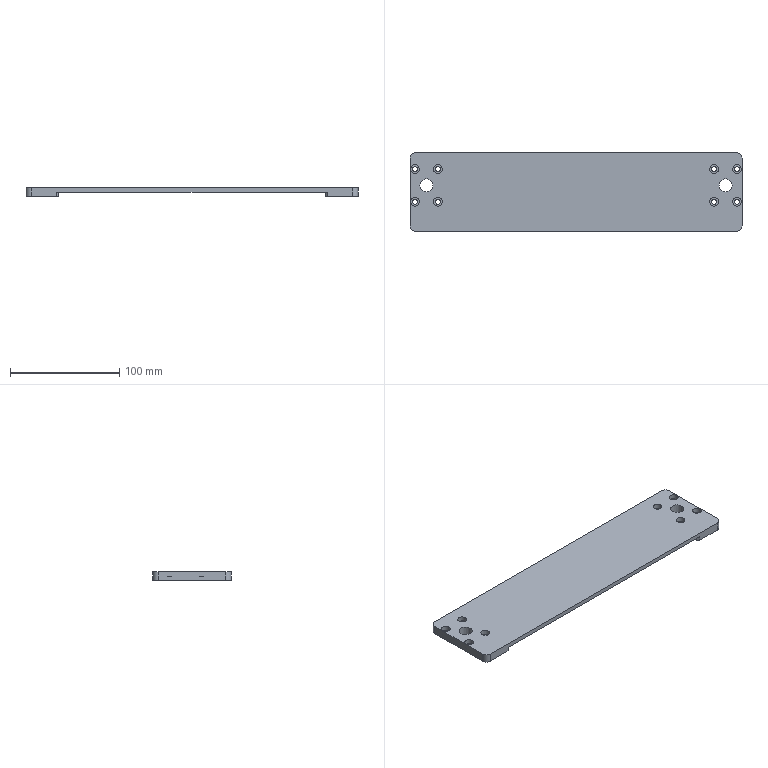Part | NX | 1 solid | 44 faces | box 304 x 72 x 8 mm | volume 100591 mm3 | plane 22 | cylinder 22 | commonest cylinder face diameters 4.5 x8 8 x8 10 x4 12 x2
STEP:
#1=CARTESIAN_POINT('',(151.5,-9.,-0.4));
#2=VERTEX_POINT('',#1);
#3=CARTESIAN_POINT('',(147.5,-9.,-0.4));
#4=DIRECTION('',(0.,0.,1.));
#5=DIRECTION('',(1.,0.,0.));
#6=AXIS2_PLACEMENT_3D('',#3,#4,#5);
#7=CIRCLE('',#6,4.);
#8=EDGE_CURVE('',#2,#2,#7,.T.);
#9=ORIENTED_EDGE('',*,*,#8,.T.);
#10=EDGE_LOOP('',(#9));
#11=FACE_BOUND('',#10,.T.);
#12=CARTESIAN_POINT('',(149.75,-9.,-0.4));
#13=VERTEX_POINT('',#12);
#14=CARTESIAN_POINT('',(147.5,-9.,-0.4));
#15=DIRECTION('',(0.,0.,1.));
#16=DIRECTION('',(1.,0.,0.));
#17=AXIS2_PLACEMENT_3D('',#14,#15,#16);
#18=CIRCLE('',#17,2.25);
#19=EDGE_CURVE('',#13,#13,#18,.T.);
#20=ORIENTED_EDGE('',*,*,#19,.F.);
#21=EDGE_LOOP('',(#20));
#22=FACE_BOUND('',#21,.T.);
#23=CARTESIAN_POINT('',(149.75,-9.,-0.4));
#24=DIRECTION('',(0.,0.,-1.));
#25=DIRECTION('',(-1.,0.,0.));
#26=AXIS2_PLACEMENT_3D('',#23,#24,#25);
#27=PLANE('',#26);
#28=ADVANCED_FACE('',(#11,#22),#27,.F.);
#29=CARTESIAN_POINT('',(143.5,21.,-0.4));
#30=VERTEX_POINT('',#29);
#31=CARTESIAN_POINT('',(147.5,21.,-0.4));
#32=DIRECTION('',(0.,0.,1.));
#33=DIRECTION('',(-1.,0.,0.));
#34=AXIS2_PLACEMENT_3D('',#31,#32,#33);
#35=CIRCLE('',#34,4.);
#36=EDGE_CURVE('',#30,#30,#35,.T.);
#37=ORIENTED_EDGE('',*,*,#36,.T.);
#38=EDGE_LOOP('',(#37));
#39=FACE_BOUND('',#38,.T.);
#40=CARTESIAN_POINT('',(145.25,21.,-0.4));
#41=VERTEX_POINT('',#40);
#42=CARTESIAN_POINT('',(147.5,21.,-0.4));
#43=DIRECTION('',(0.,0.,1.));
#44=DIRECTION('',(-1.,0.,0.));
#45=AXIS2_PLACEMENT_3D('',#42,#43,#44);
#46=CIRCLE('',#45,2.25);
#47=EDGE_CURVE('',#41,#41,#46,.T.);
#48=ORIENTED_EDGE('',*,*,#47,.F.);
#49=EDGE_LOOP('',(#48));
#50=FACE_BOUND('',#49,.T.);
#51=CARTESIAN_POINT('',(149.75,-9.,-0.4));
#52=DIRECTION('',(0.,0.,-1.));
#53=DIRECTION('',(-1.,0.,0.));
#54=AXIS2_PLACEMENT_3D('',#51,#52,#53);
#55=PLANE('',#54);
#56=ADVANCED_FACE('',(#39,#50),#55,.F.);
#57=CARTESIAN_POINT('',(122.5,21.,-0.4));
#58=VERTEX_POINT('',#57);
#59=CARTESIAN_POINT('',(126.5,21.,-0.4));
#60=DIRECTION('',(0.,0.,1.));
#61=DIRECTION('',(-1.,0.,0.));
#62=AXIS2_PLACEMENT_3D('',#59,#60,#61);
#63=CIRCLE('',#62,4.);
#64=EDGE_CURVE('',#58,#58,#63,.T.);
#65=ORIENTED_EDGE('',*,*,#64,.T.);
#66=EDGE_LOOP('',(#65));
#67=FACE_BOUND('',#66,.T.);
#68=CARTESIAN_POINT('',(124.25,21.,-0.4));
#69=VERTEX_POINT('',#68);
#70=CARTESIAN_POINT('',(126.5,21.,-0.4));
#71=DIRECTION('',(0.,0.,1.));
#72=DIRECTION('',(-1.,0.,0.));
#73=AXIS2_PLACEMENT_3D('',#70,#71,#72);
#74=CIRCLE('',#73,2.25);
#75=EDGE_CURVE('',#69,#69,#74,.T.);
#76=ORIENTED_EDGE('',*,*,#75,.F.);
#77=EDGE_LOOP('',(#76));
#78=FACE_BOUND('',#77,.T.);
#79=CARTESIAN_POINT('',(149.75,-9.,-0.4));
#80=DIRECTION('',(0.,0.,-1.));
#81=DIRECTION('',(-1.,0.,0.));
#82=AXIS2_PLACEMENT_3D('',#79,#80,#81);
#83=PLANE('',#82);
#84=ADVANCED_FACE('',(#67,#78),#83,.F.);
#85=CARTESIAN_POINT('',(122.5,-9.,-0.4));
#86=VERTEX_POINT('',#85);
#87=CARTESIAN_POINT('',(126.5,-9.,-0.4));
#88=DIRECTION('',(0.,0.,1.));
#89=DIRECTION('',(-1.,0.,0.));
#90=AXIS2_PLACEMENT_3D('',#87,#88,#89);
#91=CIRCLE('',#90,4.);
#92=EDGE_CURVE('',#86,#86,#91,.T.);
#93=ORIENTED_EDGE('',*,*,#92,.T.);
#94=EDGE_LOOP('',(#93));
#95=FACE_BOUND('',#94,.T.);
#96=CARTESIAN_POINT('',(124.25,-9.,-0.4));
#97=VERTEX_POINT('',#96);
#98=CARTESIAN_POINT('',(126.5,-9.,-0.4));
#99=DIRECTION('',(0.,0.,1.));
#100=DIRECTION('',(-1.,0.,0.));
#101=AXIS2_PLACEMENT_3D('',#98,#99,#100);
#102=CIRCLE('',#101,2.25);
#103=EDGE_CURVE('',#97,#97,#102,.T.);
#104=ORIENTED_EDGE('',*,*,#103,.F.);
#105=EDGE_LOOP('',(#104));
#106=FACE_BOUND('',#105,.T.);
#107=CARTESIAN_POINT('',(149.75,-9.,-0.4));
#108=DIRECTION('',(0.,0.,-1.));
#109=DIRECTION('',(-1.,0.,0.));
#110=AXIS2_PLACEMENT_3D('',#107,#108,#109);
#111=PLANE('',#110);
#112=ADVANCED_FACE('',(#95,#106),#111,.F.);
#113=CARTESIAN_POINT('',(-130.5,-9.,-0.4));
#114=VERTEX_POINT('',#113);
#115=CARTESIAN_POINT('',(-126.5,-9.,-0.4));
#116=DIRECTION('',(0.,0.,1.));
#117=DIRECTION('',(-1.,0.,0.));
#118=AXIS2_PLACEMENT_3D('',#115,#116,#117);
#119=CIRCLE('',#118,4.);
#120=EDGE_CURVE('',#114,#114,#119,.T.);
#121=ORIENTED_EDGE('',*,*,#120,.T.);
#122=EDGE_LOOP('',(#121));
#123=FACE_BOUND('',#122,.T.);
#124=CARTESIAN_POINT('',(-128.75,-9.,-0.4));
#125=VERTEX_POINT('',#124);
#126=CARTESIAN_POINT('',(-126.5,-9.,-0.4));
#127=DIRECTION('',(0.,0.,1.));
#128=DIRECTION('',(-1.,0.,0.));
#129=AXIS2_PLACEMENT_3D('',#126,#127,#128);
#130=CIRCLE('',#129,2.25);
#131=EDGE_CURVE('',#125,#125,#130,.T.);
#132=ORIENTED_EDGE('',*,*,#131,.F.);
#133=EDGE_LOOP('',(#132));
#134=FACE_BOUND('',#133,.T.);
#135=CARTESIAN_POINT('',(149.75,-9.,-0.4));
#136=DIRECTION('',(0.,0.,-1.));
#137=DIRECTION('',(-1.,0.,0.));
#138=AXIS2_PLACEMENT_3D('',#135,#136,#137);
#139=PLANE('',#138);
#140=ADVANCED_FACE('',(#123,#134),#139,.F.);
#141=CARTESIAN_POINT('',(-130.5,21.,-0.4));
#142=VERTEX_POINT('',#141);
#143=CARTESIAN_POINT('',(-126.5,21.,-0.4));
#144=DIRECTION('',(0.,0.,1.));
#145=DIRECTION('',(-1.,0.,0.));
#146=AXIS2_PLACEMENT_3D('',#143,#144,#145);
#147=CIRCLE('',#146,4.);
#148=EDGE_CURVE('',#142,#142,#147,.T.);
#149=ORIENTED_EDGE('',*,*,#148,.T.);
#150=EDGE_LOOP('',(#149));
#151=FACE_BOUND('',#150,.T.);
#152=CARTESIAN_POINT('',(-128.75,21.,-0.4));
#153=VERTEX_POINT('',#152);
#154=CARTESIAN_POINT('',(-126.5,21.,-0.4));
#155=DIRECTION('',(0.,0.,1.));
#156=DIRECTION('',(-1.,0.,0.));
#157=AXIS2_PLACEMENT_3D('',#154,#155,#156);
#158=CIRCLE('',#157,2.25);
#159=EDGE_CURVE('',#153,#153,#158,.T.);
#160=ORIENTED_EDGE('',*,*,#159,.F.);
#161=EDGE_LOOP('',(#160));
#162=FACE_BOUND('',#161,.T.);
#163=CARTESIAN_POINT('',(149.75,-9.,-0.4));
#164=DIRECTION('',(0.,0.,-1.));
#165=DIRECTION('',(-1.,0.,0.));
#166=AXIS2_PLACEMENT_3D('',#163,#164,#165);
#167=PLANE('',#166);
#168=ADVANCED_FACE('',(#151,#162),#167,.F.);
#169=CARTESIAN_POINT('',(-151.5,21.,-0.4));
#170=VERTEX_POINT('',#169);
#171=CARTESIAN_POINT('',(-147.5,21.,-0.4));
#172=DIRECTION('',(0.,0.,1.));
#173=DIRECTION('',(-1.,0.,0.));
#174=AXIS2_PLACEMENT_3D('',#171,#172,#173);
#175=CIRCLE('',#174,4.);
#176=EDGE_CURVE('',#170,#170,#175,.T.);
#177=ORIENTED_EDGE('',*,*,#176,.T.);
#178=EDGE_LOOP('',(#177));
#179=FACE_BOUND('',#178,.T.);
#180=CARTESIAN_POINT('',(-149.75,21.,-0.4));
#181=VERTEX_POINT('',#180);
#182=CARTESIAN_POINT('',(-147.5,21.,-0.4));
#183=DIRECTION('',(0.,0.,1.));
#184=DIRECTION('',(-1.,0.,0.));
#185=AXIS2_PLACEMENT_3D('',#182,#183,#184);
#186=CIRCLE('',#185,2.25);
#187=EDGE_CURVE('',#181,#181,#186,.T.);
#188=ORIENTED_EDGE('',*,*,#187,.F.);
#189=EDGE_LOOP('',(#188));
#190=FACE_BOUND('',#189,.T.);
#191=CARTESIAN_POINT('',(149.75,-9.,-0.4));
#192=DIRECTION('',(0.,0.,-1.));
#193=DIRECTION('',(-1.,0.,0.));
#194=AXIS2_PLACEMENT_3D('',#191,#192,#193);
#195=PLANE('',#194);
#196=ADVANCED_FACE('',(#179,#190),#195,.F.);
#197=CARTESIAN_POINT('',(-151.5,-9.,-0.4));
#198=VERTEX_POINT('',#197);
#199=CARTESIAN_POINT('',(-147.5,-9.,-0.4));
#200=DIRECTION('',(0.,0.,1.));
#201=DIRECTION('',(-1.,0.,0.));
#202=AXIS2_PLACEMENT_3D('',#199,#200,#201);
#203=CIRCLE('',#202,4.);
#204=EDGE_CURVE('',#198,#198,#203,.T.);
#205=ORIENTED_EDGE('',*,*,#204,.T.);
#206=EDGE_LOOP('',(#205));
#207=FACE_BOUND('',#206,.T.);
#208=CARTESIAN_POINT('',(-149.75,-9.,-0.4));
#209=VERTEX_POINT('',#208);
#210=CARTESIAN_POINT('',(-147.5,-9.,-0.4));
#211=DIRECTION('',(0.,0.,1.));
#212=DIRECTION('',(-1.,0.,0.));
#213=AXIS2_PLACEMENT_3D('',#210,#211,#212);
#214=CIRCLE('',#213,2.25);
#215=EDGE_CURVE('',#209,#209,#214,.T.);
#216=ORIENTED_EDGE('',*,*,#215,.F.);
#217=EDGE_LOOP('',(#216));
#218=FACE_BOUND('',#217,.T.);
#219=CARTESIAN_POINT('',(149.75,-9.,-0.4));
#220=DIRECTION('',(0.,0.,-1.));
#221=DIRECTION('',(-1.,0.,0.));
#222=AXIS2_PLACEMENT_3D('',#219,#220,#221);
#223=PLANE('',#222);
#224=ADVANCED_FACE('',(#207,#218),#223,.F.);
#225=CARTESIAN_POINT('',(-124.,-36.,0.));
#226=VERTEX_POINT('',#225);
#227=CARTESIAN_POINT('',(-122.,-34.,0.));
#228=VERTEX_POINT('',#227);
#229=CARTESIAN_POINT('',(-122.,-34.,0.));
#230=DIRECTION('',(0.7071,0.7071,0.));
#231=VECTOR('',#230,1000.);
#232=LINE('',#229,#231);
#233=EDGE_CURVE('',#226,#228,#232,.T.);
#234=ORIENTED_EDGE('',*,*,#233,.F.);
#235=CARTESIAN_POINT('',(-124.,-36.,-4.));
#236=VERTEX_POINT('',#235);
#237=CARTESIAN_POINT('',(-124.,-36.,4.));
#238=DIRECTION('',(0.,0.,1.));
#239=VECTOR('',#238,1000.);
#240=LINE('',#237,#239);
#241=EDGE_CURVE('',#236,#226,#240,.T.);
#242=ORIENTED_EDGE('',*,*,#241,.F.);
#243=CARTESIAN_POINT('',(-122.,-34.,-4.));
#244=VERTEX_POINT('',#243);
#245=CARTESIAN_POINT('',(-122.,-34.,-4.));
#246=DIRECTION('',(-0.7071,-0.7071,0.));
#247=VECTOR('',#246,1000.);
#248=LINE('',#245,#247);
#249=EDGE_CURVE('',#244,#236,#248,.T.);
#250=ORIENTED_EDGE('',*,*,#249,.F.);
#251=CARTESIAN_POINT('',(-122.,-34.,0.));
#252=DIRECTION('',(0.,0.,-1.));
#253=VECTOR('',#252,1000.);
#254=LINE('',#251,#253);
#255=EDGE_CURVE('',#228,#244,#254,.T.);
#256=ORIENTED_EDGE('',*,*,#255,.F.);
#257=EDGE_LOOP('',(#234,#242,#250,#256));
#258=FACE_BOUND('',#257,.T.);
#259=CARTESIAN_POINT('',(-122.,-34.,0.));
#260=DIRECTION('',(-0.7071,0.7071,0.));
#261=DIRECTION('',(0.,0.,-1.));
#262=AXIS2_PLACEMENT_3D('',#259,#260,#261);
#263=PLANE('',#262);
#264=ADVANCED_FACE('',(#258),#263,.F.);
#265=CARTESIAN_POINT('',(-122.,34.,0.));
#266=VERTEX_POINT('',#265);
#267=CARTESIAN_POINT('',(-124.,36.,0.));
#268=VERTEX_POINT('',#267);
#269=CARTESIAN_POINT('',(-124.,36.,0.));
#270=DIRECTION('',(-0.7071,0.7071,0.));
#271=VECTOR('',#270,1000.);
#272=LINE('',#269,#271);
#273=EDGE_CURVE('',#266,#268,#272,.T.);
#274=ORIENTED_EDGE('',*,*,#273,.F.);
#275=CARTESIAN_POINT('',(-122.,34.,-4.));
#276=VERTEX_POINT('',#275);
#277=CARTESIAN_POINT('',(-122.,34.,0.));
#278=DIRECTION('',(0.,0.,1.));
#279=VECTOR('',#278,1000.);
#280=LINE('',#277,#279);
#281=EDGE_CURVE('',#276,#266,#280,.T.);
#282=ORIENTED_EDGE('',*,*,#281,.F.);
#283=CARTESIAN_POINT('',(-124.,36.,-4.));
#284=VERTEX_POINT('',#283);
#285=CARTESIAN_POINT('',(-124.,36.,-4.));
#286=DIRECTION('',(0.7071,-0.7071,0.));
#287=VECTOR('',#286,1000.);
#288=LINE('',#285,#287);
#289=EDGE_CURVE('',#284,#276,#288,.T.);
#290=ORIENTED_EDGE('',*,*,#289,.F.);
#291=CARTESIAN_POINT('',(-124.,36.,4.));
#292=DIRECTION('',(0.,0.,-1.));
#293=VECTOR('',#292,1000.);
#294=LINE('',#291,#293);
#295=EDGE_CURVE('',#268,#284,#294,.T.);
#296=ORIENTED_EDGE('',*,*,#295,.F.);
#297=EDGE_LOOP('',(#274,#282,#290,#296));
#298=FACE_BOUND('',#297,.T.);
#299=CARTESIAN_POINT('',(-124.,36.,4.));
#300=DIRECTION('',(-0.7071,-0.7071,0.));
#301=DIRECTION('',(0.,0.,-1.));
#302=AXIS2_PLACEMENT_3D('',#299,#300,#301);
#303=PLANE('',#302);
#304=ADVANCED_FACE('',(#298),#303,.F.);
#305=CARTESIAN_POINT('',(122.,-34.,0.));
#306=VERTEX_POINT('',#305);
#307=CARTESIAN_POINT('',(124.,-36.,0.));
#308=VERTEX_POINT('',#307);
#309=CARTESIAN_POINT('',(124.,-36.,0.));
#310=DIRECTION('',(0.7071,-0.7071,0.));
#311=VECTOR('',#310,1000.);
#312=LINE('',#309,#311);
#313=EDGE_CURVE('',#306,#308,#312,.T.);
#314=ORIENTED_EDGE('',*,*,#313,.F.);
#315=CARTESIAN_POINT('',(122.,-34.,-4.));
#316=VERTEX_POINT('',#315);
#317=CARTESIAN_POINT('',(122.,-34.,0.));
#318=DIRECTION('',(0.,0.,1.));
#319=VECTOR('',#318,1000.);
#320=LINE('',#317,#319);
#321=EDGE_CURVE('',#316,#306,#320,.T.);
#322=ORIENTED_EDGE('',*,*,#321,.F.);
#323=CARTESIAN_POINT('',(124.,-36.,-4.));
#324=VERTEX_POINT('',#323);
#325=CARTESIAN_POINT('',(124.,-36.,-4.));
#326=DIRECTION('',(-0.7071,0.7071,0.));
#327=VECTOR('',#326,1000.);
#328=LINE('',#325,#327);
#329=EDGE_CURVE('',#324,#316,#328,.T.);
#330=ORIENTED_EDGE('',*,*,#329,.F.);
#331=CARTESIAN_POINT('',(124.,-36.,4.));
#332=DIRECTION('',(0.,0.,-1.));
#333=VECTOR('',#332,1000.);
#334=LINE('',#331,#333);
#335=EDGE_CURVE('',#308,#324,#334,.T.);
#336=ORIENTED_EDGE('',*,*,#335,.F.);
#337=EDGE_LOOP('',(#314,#322,#330,#336));
#338=FACE_BOUND('',#337,.T.);
#339=CARTESIAN_POINT('',(124.,-36.,4.));
#340=DIRECTION('',(0.7071,0.7071,0.));
#341=DIRECTION('',(0.,0.,-1.));
#342=AXIS2_PLACEMENT_3D('',#339,#340,#341);
#343=PLANE('',#342);
#344=ADVANCED_FACE('',(#338),#343,.F.);
#345=CARTESIAN_POINT('',(124.,36.,0.));
#346=VERTEX_POINT('',#345);
#347=CARTESIAN_POINT('',(122.,34.,0.));
#348=VERTEX_POINT('',#347);
#349=CARTESIAN_POINT('',(122.,34.,0.));
#350=DIRECTION('',(-0.7071,-0.7071,0.));
#351=VECTOR('',#350,1000.);
#352=LINE('',#349,#351);
#353=EDGE_CURVE('',#346,#348,#352,.T.);
#354=ORIENTED_EDGE('',*,*,#353,.F.);
#355=CARTESIAN_POINT('',(124.,36.,-4.));
#356=VERTEX_POINT('',#355);
#357=CARTESIAN_POINT('',(124.,36.,4.));
#358=DIRECTION('',(0.,0.,1.));
#359=VECTOR('',#358,1000.);
#360=LINE('',#357,#359);
#361=EDGE_CURVE('',#356,#346,#360,.T.);
#362=ORIENTED_EDGE('',*,*,#361,.F.);
#363=CARTESIAN_POINT('',(122.,34.,-4.));
#364=VERTEX_POINT('',#363);
#365=CARTESIAN_POINT('',(122.,34.,-4.));
#366=DIRECTION('',(0.7071,0.7071,0.));
#367=VECTOR('',#366,1000.);
#368=LINE('',#365,#367);
#369=EDGE_CURVE('',#364,#356,#368,.T.);
#370=ORIENTED_EDGE('',*,*,#369,.F.);
#371=CARTESIAN_POINT('',(122.,34.,0.));
#372=DIRECTION('',(0.,0.,-1.));
#373=VECTOR('',#372,1000.);
#374=LINE('',#371,#373);
#375=EDGE_CURVE('',#348,#364,#374,.T.);
#376=ORIENTED_EDGE('',*,*,#375,.F.);
#377=EDGE_LOOP('',(#354,#362,#370,#376));
#378=FACE_BOUND('',#377,.T.);
#379=CARTESIAN_POINT('',(122.,34.,0.));
#380=DIRECTION('',(0.7071,-0.7071,0.));
#381=DIRECTION('',(0.,0.,-1.));
#382=AXIS2_PLACEMENT_3D('',#379,#380,#381);
#383=PLANE('',#382);
#384=ADVANCED_FACE('',(#378),#383,.F.);
#385=CARTESIAN_POINT('',(122.,-36.,0.));
#386=DIRECTION('',(-1.,0.,0.));
#387=VECTOR('',#386,1000.);
#388=LINE('',#385,#387);
#389=EDGE_CURVE('',#308,#226,#388,.T.);
#390=ORIENTED_EDGE('',*,*,#389,.T.);
#391=ORIENTED_EDGE('',*,*,#233,.T.);
#392=CARTESIAN_POINT('',(-122.,36.,0.));
#393=DIRECTION('',(0.,1.,0.));
#394=VECTOR('',#393,1000.);
#395=LINE('',#392,#394);
#396=EDGE_CURVE('',#228,#266,#395,.T.);
#397=ORIENTED_EDGE('',*,*,#396,.T.);
#398=ORIENTED_EDGE('',*,*,#273,.T.);
#399=CARTESIAN_POINT('',(122.,36.,0.));
#400=DIRECTION('',(1.,0.,0.));
#401=VECTOR('',#400,1000.);
#402=LINE('',#399,#401);
#403=EDGE_CURVE('',#268,#346,#402,.T.);
#404=ORIENTED_EDGE('',*,*,#403,.T.);
#405=ORIENTED_EDGE('',*,*,#353,.T.);
#406=CARTESIAN_POINT('',(122.,36.,0.));
#407=DIRECTION('',(0.,-1.,0.));
#408=VECTOR('',#407,1000.);
#409=LINE('',#406,#408);
#410=EDGE_CURVE('',#348,#306,#409,.T.);
#411=ORIENTED_EDGE('',*,*,#410,.T.);
#412=ORIENTED_EDGE('',*,*,#313,.T.);
#413=EDGE_LOOP('',(#390,#391,#397,#398,#404,#405,#411,#412));
#414=FACE_BOUND('',#413,.T.);
#415=CARTESIAN_POINT('',(0.,0.,0.));
#416=DIRECTION('',(0.,0.,-1.));
#417=DIRECTION('',(-1.,0.,0.));
#418=AXIS2_PLACEMENT_3D('',#415,#416,#417);
#419=PLANE('',#418);
#420=ADVANCED_FACE('',(#414),#419,.T.);
#421=ORIENTED_EDGE('',*,*,#410,.F.);
#422=ORIENTED_EDGE('',*,*,#375,.T.);
#423=CARTESIAN_POINT('',(122.,36.,-4.));
#424=DIRECTION('',(0.,-1.,0.));
#425=VECTOR('',#424,1000.);
#426=LINE('',#423,#425);
#427=EDGE_CURVE('',#364,#316,#426,.T.);
#428=ORIENTED_EDGE('',*,*,#427,.T.);
#429=ORIENTED_EDGE('',*,*,#321,.T.);
#430=EDGE_LOOP('',(#421,#422,#428,#429));
#431=FACE_BOUND('',#430,.T.);
#432=CARTESIAN_POINT('',(122.,36.,0.));
#433=DIRECTION('',(1.,0.,0.));
#434=DIRECTION('',(0.,0.,-1.));
#435=AXIS2_PLACEMENT_3D('',#432,#433,#434);
#436=PLANE('',#435);
#437=ADVANCED_FACE('',(#431),#436,.F.);
#438=CARTESIAN_POINT('',(-122.,36.,-4.));
#439=DIRECTION('',(0.,1.,0.));
#440=VECTOR('',#439,1000.);
#441=LINE('',#438,#440);
#442=EDGE_CURVE('',#244,#276,#441,.T.);
#443=ORIENTED_EDGE('',*,*,#442,.T.);
#444=ORIENTED_EDGE('',*,*,#281,.T.);
#445=ORIENTED_EDGE('',*,*,#396,.F.);
#446=ORIENTED_EDGE('',*,*,#255,.T.);
#447=EDGE_LOOP('',(#443,#444,#445,#446));
#448=FACE_BOUND('',#447,.T.);
#449=CARTESIAN_POINT('',(-122.,36.,0.));
#450=DIRECTION('',(-1.,0.,0.));
#451=DIRECTION('',(0.,0.,1.));
#452=AXIS2_PLACEMENT_3D('',#449,#450,#451);
#453=PLANE('',#452);
#454=ADVANCED_FACE('',(#448),#453,.F.);
#455=CARTESIAN_POINT('',(-147.,36.,4.));
#456=VERTEX_POINT('',#455);
#457=CARTESIAN_POINT('',(-152.,31.,4.));
#458=VERTEX_POINT('',#457);
#459=CARTESIAN_POINT('',(-147.,31.,4.));
#460=DIRECTION('',(0.,0.,1.));
#461=DIRECTION('',(1.,0.,0.));
#462=AXIS2_PLACEMENT_3D('',#459,#460,#461);
#463=CIRCLE('',#462,5.);
#464=EDGE_CURVE('',#456,#458,#463,.T.);
#465=ORIENTED_EDGE('',*,*,#464,.F.);
#466=CARTESIAN_POINT('',(-147.,36.,-4.));
#467=VERTEX_POINT('',#466);
#468=CARTESIAN_POINT('',(-147.,36.,4.));
#469=DIRECTION('',(0.,0.,1.));
#470=VECTOR('',#469,1000.);
#471=LINE('',#468,#470);
#472=EDGE_CURVE('',#467,#456,#471,.T.);
#473=ORIENTED_EDGE('',*,*,#472,.F.);
#474=CARTESIAN_POINT('',(-152.,31.,-4.));
#475=VERTEX_POINT('',#474);
#476=CARTESIAN_POINT('',(-147.,31.,-4.));
#477=DIRECTION('',(0.,0.,-1.));
#478=DIRECTION('',(1.,0.,0.));
#479=AXIS2_PLACEMENT_3D('',#476,#477,#478);
#480=CIRCLE('',#479,5.);
#481=EDGE_CURVE('',#475,#467,#480,.T.);
#482=ORIENTED_EDGE('',*,*,#481,.F.);
#483=CARTESIAN_POINT('',(-152.,31.,4.));
#484=DIRECTION('',(0.,0.,-1.));
#485=VECTOR('',#484,1000.);
#486=LINE('',#483,#485);
#487=EDGE_CURVE('',#458,#475,#486,.T.);
#488=ORIENTED_EDGE('',*,*,#487,.F.);
#489=EDGE_LOOP('',(#465,#473,#482,#488));
#490=FACE_BOUND('',#489,.T.);
#491=CARTESIAN_POINT('',(-147.,31.,4.));
#492=DIRECTION('',(0.,0.,-1.));
#493=DIRECTION('',(-1.,0.,0.));
#494=AXIS2_PLACEMENT_3D('',#491,#492,#493);
#495=CYLINDRICAL_SURFACE('',#494,5.);
#496=ADVANCED_FACE('',(#490),#495,.T.);
#497=CARTESIAN_POINT('',(-152.,-31.,4.));
#498=VERTEX_POINT('',#497);
#499=CARTESIAN_POINT('',(-147.,-36.,4.));
#500=VERTEX_POINT('',#499);
#501=CARTESIAN_POINT('',(-147.,-31.,4.));
#502=DIRECTION('',(0.,0.,1.));
#503=DIRECTION('',(1.,0.,0.));
#504=AXIS2_PLACEMENT_3D('',#501,#502,#503);
#505=CIRCLE('',#504,5.);
#506=EDGE_CURVE('',#498,#500,#505,.T.);
#507=ORIENTED_EDGE('',*,*,#506,.F.);
#508=CARTESIAN_POINT('',(-152.,-31.,-4.));
#509=VERTEX_POINT('',#508);
#510=CARTESIAN_POINT('',(-152.,-31.,4.));
#511=DIRECTION('',(0.,0.,1.));
#512=VECTOR('',#511,1000.);
#513=LINE('',#510,#512);
#514=EDGE_CURVE('',#509,#498,#513,.T.);
#515=ORIENTED_EDGE('',*,*,#514,.F.);
#516=CARTESIAN_POINT('',(-147.,-36.,-4.));
#517=VERTEX_POINT('',#516);
#518=CARTESIAN_POINT('',(-147.,-31.,-4.));
#519=DIRECTION('',(0.,0.,-1.));
#520=DIRECTION('',(1.,0.,0.));
#521=AXIS2_PLACEMENT_3D('',#518,#519,#520);
#522=CIRCLE('',#521,5.);
#523=EDGE_CURVE('',#517,#509,#522,.T.);
#524=ORIENTED_EDGE('',*,*,#523,.F.);
#525=CARTESIAN_POINT('',(-147.,-36.,4.));
#526=DIRECTION('',(0.,0.,-1.));
#527=VECTOR('',#526,1000.);
#528=LINE('',#525,#527);
#529=EDGE_CURVE('',#500,#517,#528,.T.);
#530=ORIENTED_EDGE('',*,*,#529,.F.);
#531=EDGE_LOOP('',(#507,#515,#524,#530));
#532=FACE_BOUND('',#531,.T.);
#533=CARTESIAN_POINT('',(-147.,-31.,4.));
#534=DIRECTION('',(0.,0.,-1.));
#535=DIRECTION('',(-1.,0.,0.));
#536=AXIS2_PLACEMENT_3D('',#533,#534,#535);
#537=CYLINDRICAL_SURFACE('',#536,5.);
#538=ADVANCED_FACE('',(#532),#537,.T.);
#539=CARTESIAN_POINT('',(152.,31.,4.));
#540=VERTEX_POINT('',#539);
#541=CARTESIAN_POINT('',(147.,36.,4.));
#542=VERTEX_POINT('',#541);
#543=CARTESIAN_POINT('',(147.,31.,4.));
#544=DIRECTION('',(0.,0.,1.));
#545=DIRECTION('',(1.,0.,0.));
#546=AXIS2_PLACEMENT_3D('',#543,#544,#545);
#547=CIRCLE('',#546,5.);
#548=EDGE_CURVE('',#540,#542,#547,.T.);
#549=ORIENTED_EDGE('',*,*,#548,.F.);
#550=CARTESIAN_POINT('',(152.,31.,-4.));
#551=VERTEX_POINT('',#550);
#552=CARTESIAN_POINT('',(152.,31.,4.));
#553=DIRECTION('',(0.,0.,1.));
#554=VECTOR('',#553,1000.);
#555=LINE('',#552,#554);
#556=EDGE_CURVE('',#551,#540,#555,.T.);
#557=ORIENTED_EDGE('',*,*,#556,.F.);
#558=CARTESIAN_POINT('',(147.,36.,-4.));
#559=VERTEX_POINT('',#558);
#560=CARTESIAN_POINT('',(147.,31.,-4.));
#561=DIRECTION('',(0.,0.,-1.));
#562=DIRECTION('',(1.,0.,0.));
#563=AXIS2_PLACEMENT_3D('',#560,#561,#562);
#564=CIRCLE('',#563,5.);
#565=EDGE_CURVE('',#559,#551,#564,.T.);
#566=ORIENTED_EDGE('',*,*,#565,.F.);
#567=CARTESIAN_POINT('',(147.,36.,4.));
#568=DIRECTION('',(0.,0.,-1.));
#569=VECTOR('',#568,1000.);
#570=LINE('',#567,#569);
#571=EDGE_CURVE('',#542,#559,#570,.T.);
#572=ORIENTED_EDGE('',*,*,#571,.F.);
#573=EDGE_LOOP('',(#549,#557,#566,#572));
#574=FACE_BOUND('',#573,.T.);
#575=CARTESIAN_POINT('',(147.,31.,4.));
#576=DIRECTION('',(0.,0.,-1.));
#577=DIRECTION('',(-1.,0.,0.));
#578=AXIS2_PLACEMENT_3D('',#575,#576,#577);
#579=CYLINDRICAL_SURFACE('',#578,5.);
#580=ADVANCED_FACE('',(#574),#579,.T.);
#581=CARTESIAN_POINT('',(147.,-36.,4.));
#582=VERTEX_POINT('',#581);
#583=CARTESIAN_POINT('',(152.,-31.,4.));
#584=VERTEX_POINT('',#583);
#585=CARTESIAN_POINT('',(147.,-31.,4.));
#586=DIRECTION('',(0.,0.,1.));
#587=DIRECTION('',(1.,0.,0.));
#588=AXIS2_PLACEMENT_3D('',#585,#586,#587);
#589=CIRCLE('',#588,5.);
#590=EDGE_CURVE('',#582,#584,#589,.T.);
#591=ORIENTED_EDGE('',*,*,#590,.F.);
#592=CARTESIAN_POINT('',(147.,-36.,-4.));
#593=VERTEX_POINT('',#592);
#594=CARTESIAN_POINT('',(147.,-36.,4.));
#595=DIRECTION('',(0.,0.,1.));
#596=VECTOR('',#595,1000.);
#597=LINE('',#594,#596);
#598=EDGE_CURVE('',#593,#582,#597,.T.);
#599=ORIENTED_EDGE('',*,*,#598,.F.);
#600=CARTESIAN_POINT('',(152.,-31.,-4.));
#601=VERTEX_POINT('',#600);
#602=CARTESIAN_POINT('',(147.,-31.,-4.));
#603=DIRECTION('',(0.,0.,-1.));
#604=DIRECTION('',(1.,0.,0.));
#605=AXIS2_PLACEMENT_3D('',#602,#603,#604);
#606=CIRCLE('',#605,5.);
#607=EDGE_CURVE('',#601,#593,#606,.T.);
#608=ORIENTED_EDGE('',*,*,#607,.F.);
#609=CARTESIAN_POINT('',(152.,-31.,4.));
#610=DIRECTION('',(0.,0.,-1.));
#611=VECTOR('',#610,1000.);
#612=LINE('',#609,#611);
#613=EDGE_CURVE('',#584,#601,#612,.T.);
#614=ORIENTED_EDGE('',*,*,#613,.F.);
#615=EDGE_LOOP('',(#591,#599,#608,#614));
#616=FACE_BOUND('',#615,.T.);
#617=CARTESIAN_POINT('',(147.,-31.,4.));
#618=DIRECTION('',(0.,0.,-1.));
#619=DIRECTION('',(-1.,0.,0.));
#620=AXIS2_PLACEMENT_3D('',#617,#618,#619);
#621=CYLINDRICAL_SURFACE('',#620,5.);
#622=ADVANCED_FACE('',(#616),#621,.T.);
#623=ORIENTED_EDGE('',*,*,#427,.F.);
#624=ORIENTED_EDGE('',*,*,#369,.T.);
#625=CARTESIAN_POINT('',(152.,36.,-4.));
#626=DIRECTION('',(-1.,0.,0.));
#627=VECTOR('',#626,1000.);
#628=LINE('',#625,#627);
#629=EDGE_CURVE('',#559,#356,#628,.T.);
#630=ORIENTED_EDGE('',*,*,#629,.F.);
#631=ORIENTED_EDGE('',*,*,#565,.T.);
#632=CARTESIAN_POINT('',(152.,-36.,-4.));
#633=DIRECTION('',(0.,1.,0.));
#634=VECTOR('',#633,1000.);
#635=LINE('',#632,#634);
#636=EDGE_CURVE('',#601,#551,#635,.T.);
#637=ORIENTED_EDGE('',*,*,#636,.F.);
#638=ORIENTED_EDGE('',*,*,#607,.T.);
#639=CARTESIAN_POINT('',(152.,-36.,-4.));
#640=DIRECTION('',(1.,0.,0.));
#641=VECTOR('',#640,1000.);
#642=LINE('',#639,#641);
#643=EDGE_CURVE('',#324,#593,#642,.T.);
#644=ORIENTED_EDGE('',*,*,#643,.F.);
#645=ORIENTED_EDGE('',*,*,#329,.T.);
#646=EDGE_LOOP('',(#623,#624,#630,#631,#637,#638,#644,#645));
#647=FACE_BOUND('',#646,.T.);
#648=CARTESIAN_POINT('',(143.,6.,-4.));
#649=VERTEX_POINT('',#648);
#650=CARTESIAN_POINT('',(137.,6.,-4.));
#651=DIRECTION('',(0.,0.,1.));
#652=DIRECTION('',(1.,0.,0.));
#653=AXIS2_PLACEMENT_3D('',#650,#651,#652);
#654=CIRCLE('',#653,6.);
#655=EDGE_CURVE('',#649,#649,#654,.T.);
#656=ORIENTED_EDGE('',*,*,#655,.T.);
#657=EDGE_LOOP('',(#656));
#658=FACE_BOUND('',#657,.T.);
#659=CARTESIAN_POINT('',(128.75,-9.,-4.));
#660=VERTEX_POINT('',#659);
#661=CARTESIAN_POINT('',(126.5,-9.,-4.));
#662=DIRECTION('',(0.,0.,1.));
#663=DIRECTION('',(1.,0.,0.));
#664=AXIS2_PLACEMENT_3D('',#661,#662,#663);
#665=CIRCLE('',#664,2.25);
#666=EDGE_CURVE('',#660,#660,#665,.T.);
#667=ORIENTED_EDGE('',*,*,#666,.T.);
#668=EDGE_LOOP('',(#667));
#669=FACE_BOUND('',#668,.T.);
#670=CARTESIAN_POINT('',(128.75,21.,-4.));
#671=VERTEX_POINT('',#670);
#672=CARTESIAN_POINT('',(126.5,21.,-4.));
#673=DIRECTION('',(0.,0.,1.));
#674=DIRECTION('',(1.,0.,0.));
#675=AXIS2_PLACEMENT_3D('',#672,#673,#674);
#676=CIRCLE('',#675,2.25);
#677=EDGE_CURVE('',#671,#671,#676,.T.);
#678=ORIENTED_EDGE('',*,*,#677,.T.);
#679=EDGE_LOOP('',(#678));
#680=FACE_BOUND('',#679,.T.);
#681=CARTESIAN_POINT('',(149.75,21.,-4.));
#682=VERTEX_POINT('',#681);
#683=CARTESIAN_POINT('',(147.5,21.,-4.));
#684=DIRECTION('',(0.,0.,1.));
#685=DIRECTION('',(1.,0.,0.));
#686=AXIS2_PLACEMENT_3D('',#683,#684,#685);
#687=CIRCLE('',#686,2.25);
#688=EDGE_CURVE('',#682,#682,#687,.T.);
#689=ORIENTED_EDGE('',*,*,#688,.T.);
#690=EDGE_LOOP('',(#689));
#691=FACE_BOUND('',#690,.T.);
#692=CARTESIAN_POINT('',(149.75,-9.,-4.));
#693=VERTEX_POINT('',#692);
#694=CARTESIAN_POINT('',(147.5,-9.,-4.));
#695=DIRECTION('',(0.,0.,1.));
#696=DIRECTION('',(1.,0.,0.));
#697=AXIS2_PLACEMENT_3D('',#694,#695,#696);
#698=CIRCLE('',#697,2.25);
#699=EDGE_CURVE('',#693,#693,#698,.T.);
#700=ORIENTED_EDGE('',*,*,#699,.T.);
#701=EDGE_LOOP('',(#700));
#702=FACE_BOUND('',#701,.T.);
#703=CARTESIAN_POINT('',(0.,0.,-4.));
#704=DIRECTION('',(0.,0.,1.));
#705=DIRECTION('',(1.,0.,0.));
#706=AXIS2_PLACEMENT_3D('',#703,#704,#705);
#707=PLANE('',#706);
#708=ADVANCED_FACE('',(#647,#658,#669,#680,#691,#702),#707,.F.);
#709=CARTESIAN_POINT('',(152.,-36.,4.));
#710=DIRECTION('',(1.,0.,0.));
#711=VECTOR('',#710,1000.);
#712=LINE('',#709,#711);
#713=EDGE_CURVE('',#500,#582,#712,.T.);
#714=ORIENTED_EDGE('',*,*,#713,.T.);
#715=ORIENTED_EDGE('',*,*,#590,.T.);
#716=CARTESIAN_POINT('',(152.,-36.,4.));
#717=DIRECTION('',(0.,1.,0.));
#718=VECTOR('',#717,1000.);
#719=LINE('',#716,#718);
#720=EDGE_CURVE('',#584,#540,#719,.T.);
#721=ORIENTED_EDGE('',*,*,#720,.T.);
#722=ORIENTED_EDGE('',*,*,#548,.T.);
#723=CARTESIAN_POINT('',(152.,36.,4.));
#724=DIRECTION('',(-1.,0.,0.));
#725=VECTOR('',#724,1000.);
#726=LINE('',#723,#725);
#727=EDGE_CURVE('',#542,#456,#726,.T.);
#728=ORIENTED_EDGE('',*,*,#727,.T.);
#729=ORIENTED_EDGE('',*,*,#464,.T.);
#730=CARTESIAN_POINT('',(-152.,-36.,4.));
#731=DIRECTION('',(0.,-1.,0.));
#732=VECTOR('',#731,1000.);
#733=LINE('',#730,#732);
#734=EDGE_CURVE('',#458,#498,#733,.T.);
#735=ORIENTED_EDGE('',*,*,#734,.T.);
#736=ORIENTED_EDGE('',*,*,#506,.T.);
#737=EDGE_LOOP('',(#714,#715,#721,#722,#728,#729,#735,#736));
#738=FACE_BOUND('',#737,.T.);
#739=CARTESIAN_POINT('',(-143.,6.,4.));
#740=VERTEX_POINT('',#739);
#741=CARTESIAN_POINT('',(-137.,6.,4.));
#742=DIRECTION('',(0.,0.,1.));
#743=DIRECTION('',(-1.,0.,0.));
#744=AXIS2_PLACEMENT_3D('',#741,#742,#743);
#745=CIRCLE('',#744,6.);
#746=EDGE_CURVE('',#740,#740,#745,.T.);
#747=ORIENTED_EDGE('',*,*,#746,.F.);
#748=EDGE_LOOP('',(#747));
#749=FACE_BOUND('',#748,.T.);
#750=CARTESIAN_POINT('',(143.,6.,4.));
#751=VERTEX_POINT('',#750);
#752=CARTESIAN_POINT('',(137.,6.,4.));
#753=DIRECTION('',(0.,0.,1.));
#754=DIRECTION('',(1.,0.,0.));
#755=AXIS2_PLACEMENT_3D('',#752,#753,#754);
#756=CIRCLE('',#755,6.);
#757=EDGE_CURVE('',#751,#751,#756,.T.);
#758=ORIENTED_EDGE('',*,*,#757,.F.);
#759=EDGE_LOOP('',(#758));
#760=FACE_BOUND('',#759,.T.);
#761=CARTESIAN_POINT('',(-143.5,-9.,4.));
#762=VERTEX_POINT('',#761);
#763=CARTESIAN_POINT('',(-147.5,-9.,4.));
#764=DIRECTION('',(0.,0.,1.));
#765=DIRECTION('',(1.,0.,0.));
#766=AXIS2_PLACEMENT_3D('',#763,#764,#765);
#767=CIRCLE('',#766,4.);
#768=EDGE_CURVE('',#762,#762,#767,.T.);
#769=ORIENTED_EDGE('',*,*,#768,.F.);
#770=EDGE_LOOP('',(#769));
#771=FACE_BOUND('',#770,.T.);
#772=CARTESIAN_POINT('',(-143.5,21.,4.));
#773=VERTEX_POINT('',#772);
#774=CARTESIAN_POINT('',(-147.5,21.,4.));
#775=DIRECTION('',(0.,0.,1.));
#776=DIRECTION('',(1.,0.,0.));
#777=AXIS2_PLACEMENT_3D('',#774,#775,#776);
#778=CIRCLE('',#777,4.);
#779=EDGE_CURVE('',#773,#773,#778,.T.);
#780=ORIENTED_EDGE('',*,*,#779,.F.);
#781=EDGE_LOOP('',(#780));
#782=FACE_BOUND('',#781,.T.);
#783=CARTESIAN_POINT('',(-122.5,21.,4.));
#784=VERTEX_POINT('',#783);
#785=CARTESIAN_POINT('',(-126.5,21.,4.));
#786=DIRECTION('',(0.,0.,1.));
#787=DIRECTION('',(1.,0.,0.));
#788=AXIS2_PLACEMENT_3D('',#785,#786,#787);
#789=CIRCLE('',#788,4.);
#790=EDGE_CURVE('',#784,#784,#789,.T.);
#791=ORIENTED_EDGE('',*,*,#790,.F.);
#792=EDGE_LOOP('',(#791));
#793=FACE_BOUND('',#792,.T.);
#794=CARTESIAN_POINT('',(-122.5,-9.,4.));
#795=VERTEX_POINT('',#794);
#796=CARTESIAN_POINT('',(-126.5,-9.,4.));
#797=DIRECTION('',(0.,0.,1.));
#798=DIRECTION('',(1.,0.,0.));
#799=AXIS2_PLACEMENT_3D('',#796,#797,#798);
#800=CIRCLE('',#799,4.);
#801=EDGE_CURVE('',#795,#795,#800,.T.);
#802=ORIENTED_EDGE('',*,*,#801,.F.);
#803=EDGE_LOOP('',(#802));
#804=FACE_BOUND('',#803,.T.);
#805=CARTESIAN_POINT('',(130.5,-9.,4.));
#806=VERTEX_POINT('',#805);
#807=CARTESIAN_POINT('',(126.5,-9.,4.));
#808=DIRECTION('',(0.,0.,1.));
#809=DIRECTION('',(1.,0.,0.));
#810=AXIS2_PLACEMENT_3D('',#807,#808,#809);
#811=CIRCLE('',#810,4.);
#812=EDGE_CURVE('',#806,#806,#811,.T.);
#813=ORIENTED_EDGE('',*,*,#812,.F.);
#814=EDGE_LOOP('',(#813));
#815=FACE_BOUND('',#814,.T.);
#816=CARTESIAN_POINT('',(130.5,21.,4.));
#817=VERTEX_POINT('',#816);
#818=CARTESIAN_POINT('',(126.5,21.,4.));
#819=DIRECTION('',(0.,0.,1.));
#820=DIRECTION('',(1.,0.,0.));
#821=AXIS2_PLACEMENT_3D('',#818,#819,#820);
#822=CIRCLE('',#821,4.);
#823=EDGE_CURVE('',#817,#817,#822,.T.);
#824=ORIENTED_EDGE('',*,*,#823,.F.);
#825=EDGE_LOOP('',(#824));
#826=FACE_BOUND('',#825,.T.);
#827=CARTESIAN_POINT('',(151.5,21.,4.));
#828=VERTEX_POINT('',#827);
#829=CARTESIAN_POINT('',(147.5,21.,4.));
#830=DIRECTION('',(0.,0.,1.));
#831=DIRECTION('',(1.,0.,0.));
#832=AXIS2_PLACEMENT_3D('',#829,#830,#831);
#833=CIRCLE('',#832,4.);
#834=EDGE_CURVE('',#828,#828,#833,.T.);
#835=ORIENTED_EDGE('',*,*,#834,.F.);
#836=EDGE_LOOP('',(#835));
#837=FACE_BOUND('',#836,.T.);
#838=CARTESIAN_POINT('',(151.5,-9.,4.));
#839=VERTEX_POINT('',#838);
#840=CARTESIAN_POINT('',(147.5,-9.,4.));
#841=DIRECTION('',(0.,0.,1.));
#842=DIRECTION('',(1.,0.,0.));
#843=AXIS2_PLACEMENT_3D('',#840,#841,#842);
#844=CIRCLE('',#843,4.);
#845=EDGE_CURVE('',#839,#839,#844,.T.);
#846=ORIENTED_EDGE('',*,*,#845,.F.);
#847=EDGE_LOOP('',(#846));
#848=FACE_BOUND('',#847,.T.);
#849=CARTESIAN_POINT('',(0.,0.,4.));
#850=DIRECTION('',(0.,0.,1.));
#851=DIRECTION('',(1.,0.,0.));
#852=AXIS2_PLACEMENT_3D('',#849,#850,#851);
#853=PLANE('',#852);
#854=ADVANCED_FACE('',(#738,#749,#760,#771,#782,#793,#804,#815,#826,#837,#848),#853,.T.);
#855=ORIENTED_EDGE('',*,*,#629,.T.);
#856=ORIENTED_EDGE('',*,*,#361,.T.);
#857=ORIENTED_EDGE('',*,*,#403,.F.);
#858=ORIENTED_EDGE('',*,*,#295,.T.);
#859=CARTESIAN_POINT('',(152.,36.,-4.));
#860=DIRECTION('',(-1.,0.,0.));
#861=VECTOR('',#860,1000.);
#862=LINE('',#859,#861);
#863=EDGE_CURVE('',#284,#467,#862,.T.);
#864=ORIENTED_EDGE('',*,*,#863,.T.);
#865=ORIENTED_EDGE('',*,*,#472,.T.);
#866=ORIENTED_EDGE('',*,*,#727,.F.);
#867=ORIENTED_EDGE('',*,*,#571,.T.);
#868=EDGE_LOOP('',(#855,#856,#857,#858,#864,#865,#866,#867));
#869=FACE_BOUND('',#868,.T.);
#870=CARTESIAN_POINT('',(152.,36.,4.));
#871=DIRECTION('',(0.,-1.,0.));
#872=DIRECTION('',(1.,0.,0.));
#873=AXIS2_PLACEMENT_3D('',#870,#871,#872);
#874=PLANE('',#873);
#875=ADVANCED_FACE('',(#869),#874,.F.);
#876=ORIENTED_EDGE('',*,*,#720,.F.);
#877=ORIENTED_EDGE('',*,*,#613,.T.);
#878=ORIENTED_EDGE('',*,*,#636,.T.);
#879=ORIENTED_EDGE('',*,*,#556,.T.);
#880=EDGE_LOOP('',(#876,#877,#878,#879));
#881=FACE_BOUND('',#880,.T.);
#882=CARTESIAN_POINT('',(152.,-36.,4.));
#883=DIRECTION('',(-1.,0.,0.));
#884=DIRECTION('',(0.,0.,1.));
#885=AXIS2_PLACEMENT_3D('',#882,#883,#884);
#886=PLANE('',#885);
#887=ADVANCED_FACE('',(#881),#886,.F.);
#888=ORIENTED_EDGE('',*,*,#389,.F.);
#889=ORIENTED_EDGE('',*,*,#335,.T.);
#890=ORIENTED_EDGE('',*,*,#643,.T.);
#891=ORIENTED_EDGE('',*,*,#598,.T.);
#892=ORIENTED_EDGE('',*,*,#713,.F.);
#893=ORIENTED_EDGE('',*,*,#529,.T.);
#894=CARTESIAN_POINT('',(152.,-36.,-4.));
#895=DIRECTION('',(1.,0.,0.));
#896=VECTOR('',#895,1000.);
#897=LINE('',#894,#896);
#898=EDGE_CURVE('',#517,#236,#897,.T.);
#899=ORIENTED_EDGE('',*,*,#898,.T.);
#900=ORIENTED_EDGE('',*,*,#241,.T.);
#901=EDGE_LOOP('',(#888,#889,#890,#891,#892,#893,#899,#900));
#902=FACE_BOUND('',#901,.T.);
#903=CARTESIAN_POINT('',(152.,-36.,4.));
#904=DIRECTION('',(0.,1.,0.));
#905=DIRECTION('',(-1.,0.,0.));
#906=AXIS2_PLACEMENT_3D('',#903,#904,#905);
#907=PLANE('',#906);
#908=ADVANCED_FACE('',(#902),#907,.F.);
#909=CARTESIAN_POINT('',(-152.,-36.,-4.));
#910=DIRECTION('',(0.,-1.,0.));
#911=VECTOR('',#910,1000.);
#912=LINE('',#909,#911);
#913=EDGE_CURVE('',#475,#509,#912,.T.);
#914=ORIENTED_EDGE('',*,*,#913,.T.);
#915=ORIENTED_EDGE('',*,*,#514,.T.);
#916=ORIENTED_EDGE('',*,*,#734,.F.);
#917=ORIENTED_EDGE('',*,*,#487,.T.);
#918=EDGE_LOOP('',(#914,#915,#916,#917));
#919=FACE_BOUND('',#918,.T.);
#920=CARTESIAN_POINT('',(-152.,-36.,4.));
#921=DIRECTION('',(1.,0.,0.));
#922=DIRECTION('',(0.,0.,-1.));
#923=AXIS2_PLACEMENT_3D('',#920,#921,#922);
#924=PLANE('',#923);
#925=ADVANCED_FACE('',(#919),#924,.F.);
#926=ORIENTED_EDGE('',*,*,#863,.F.);
#927=ORIENTED_EDGE('',*,*,#289,.T.);
#928=ORIENTED_EDGE('',*,*,#442,.F.);
#929=ORIENTED_EDGE('',*,*,#249,.T.);
#930=ORIENTED_EDGE('',*,*,#898,.F.);
#931=ORIENTED_EDGE('',*,*,#523,.T.);
#932=ORIENTED_EDGE('',*,*,#913,.F.);
#933=ORIENTED_EDGE('',*,*,#481,.T.);
#934=EDGE_LOOP('',(#926,#927,#928,#929,#930,#931,#932,#933));
#935=FACE_BOUND('',#934,.T.);
#936=CARTESIAN_POINT('',(-143.,6.,-4.));
#937=VERTEX_POINT('',#936);
#938=CARTESIAN_POINT('',(-137.,6.,-4.));
#939=DIRECTION('',(0.,0.,1.));
#940=DIRECTION('',(-1.,0.,0.));
#941=AXIS2_PLACEMENT_3D('',#938,#939,#940);
#942=CIRCLE('',#941,6.);
#943=EDGE_CURVE('',#937,#937,#942,.T.);
#944=ORIENTED_EDGE('',*,*,#943,.T.);
#945=EDGE_LOOP('',(#944));
#946=FACE_BOUND('',#945,.T.);
#947=CARTESIAN_POINT('',(-145.25,-9.,-4.));
#948=VERTEX_POINT('',#947);
#949=CARTESIAN_POINT('',(-147.5,-9.,-4.));
#950=DIRECTION('',(0.,0.,1.));
#951=DIRECTION('',(1.,0.,0.));
#952=AXIS2_PLACEMENT_3D('',#949,#950,#951);
#953=CIRCLE('',#952,2.25);
#954=EDGE_CURVE('',#948,#948,#953,.T.);
#955=ORIENTED_EDGE('',*,*,#954,.T.);
#956=EDGE_LOOP('',(#955));
#957=FACE_BOUND('',#956,.T.);
#958=CARTESIAN_POINT('',(-145.25,21.,-4.));
#959=VERTEX_POINT('',#958);
#960=CARTESIAN_POINT('',(-147.5,21.,-4.));
#961=DIRECTION('',(0.,0.,1.));
#962=DIRECTION('',(1.,0.,0.));
#963=AXIS2_PLACEMENT_3D('',#960,#961,#962);
#964=CIRCLE('',#963,2.25);
#965=EDGE_CURVE('',#959,#959,#964,.T.);
#966=ORIENTED_EDGE('',*,*,#965,.T.);
#967=EDGE_LOOP('',(#966));
#968=FACE_BOUND('',#967,.T.);
#969=CARTESIAN_POINT('',(-124.25,21.,-4.));
#970=VERTEX_POINT('',#969);
#971=CARTESIAN_POINT('',(-126.5,21.,-4.));
#972=DIRECTION('',(0.,0.,1.));
#973=DIRECTION('',(1.,0.,0.));
#974=AXIS2_PLACEMENT_3D('',#971,#972,#973);
#975=CIRCLE('',#974,2.25);
#976=EDGE_CURVE('',#970,#970,#975,.T.);
#977=ORIENTED_EDGE('',*,*,#976,.T.);
#978=EDGE_LOOP('',(#977));
#979=FACE_BOUND('',#978,.T.);
#980=CARTESIAN_POINT('',(-124.25,-9.,-4.));
#981=VERTEX_POINT('',#980);
#982=CARTESIAN_POINT('',(-126.5,-9.,-4.));
#983=DIRECTION('',(0.,0.,1.));
#984=DIRECTION('',(1.,0.,0.));
#985=AXIS2_PLACEMENT_3D('',#982,#983,#984);
#986=CIRCLE('',#985,2.25);
#987=EDGE_CURVE('',#981,#981,#986,.T.);
#988=ORIENTED_EDGE('',*,*,#987,.T.);
#989=EDGE_LOOP('',(#988));
#990=FACE_BOUND('',#989,.T.);
#991=CARTESIAN_POINT('',(0.,0.,-4.));
#992=DIRECTION('',(0.,0.,1.));
#993=DIRECTION('',(1.,0.,0.));
#994=AXIS2_PLACEMENT_3D('',#991,#992,#993);
#995=PLANE('',#994);
#996=ADVANCED_FACE('',(#935,#946,#957,#968,#979,#990),#995,.F.);
#997=ORIENTED_EDGE('',*,*,#943,.F.);
#998=EDGE_LOOP('',(#997));
#999=FACE_BOUND('',#998,.T.);
#1000=ORIENTED_EDGE('',*,*,#746,.T.);
#1001=EDGE_LOOP('',(#1000));
#1002=FACE_BOUND('',#1001,.T.);
#1003=CARTESIAN_POINT('',(-137.,6.,-4.));
#1004=DIRECTION('',(0.,0.,1.));
#1005=DIRECTION('',(1.,0.,0.));
#1006=AXIS2_PLACEMENT_3D('',#1003,#1004,#1005);
#1007=CYLINDRICAL_SURFACE('',#1006,6.);
#1008=ADVANCED_FACE('',(#999,#1002),#1007,.F.);
#1009=ORIENTED_EDGE('',*,*,#655,.F.);
#1010=EDGE_LOOP('',(#1009));
#1011=FACE_BOUND('',#1010,.T.);
#1012=ORIENTED_EDGE('',*,*,#757,.T.);
#1013=EDGE_LOOP('',(#1012));
#1014=FACE_BOUND('',#1013,.T.);
#1015=CARTESIAN_POINT('',(137.,6.,-4.));
#1016=DIRECTION('',(0.,0.,1.));
#1017=DIRECTION('',(1.,0.,0.));
#1018=AXIS2_PLACEMENT_3D('',#1015,#1016,#1017);
#1019=CYLINDRICAL_SURFACE('',#1018,6.);
#1020=ADVANCED_FACE('',(#1011,#1014),#1019,.F.);
#1021=ORIENTED_EDGE('',*,*,#954,.F.);
#1022=EDGE_LOOP('',(#1021));
#1023=FACE_BOUND('',#1022,.T.);
#1024=ORIENTED_EDGE('',*,*,#215,.T.);
#1025=EDGE_LOOP('',(#1024));
#1026=FACE_BOUND('',#1025,.T.);
#1027=CARTESIAN_POINT('',(-147.5,-9.,4.));
#1028=DIRECTION('',(0.,0.,1.));
#1029=DIRECTION('',(1.,0.,0.));
#1030=AXIS2_PLACEMENT_3D('',#1027,#1028,#1029);
#1031=CYLINDRICAL_SURFACE('',#1030,2.25);
#1032=ADVANCED_FACE('',(#1023,#1026),#1031,.F.);
#1033=ORIENTED_EDGE('',*,*,#204,.F.);
#1034=EDGE_LOOP('',(#1033));
#1035=FACE_BOUND('',#1034,.T.);
#1036=ORIENTED_EDGE('',*,*,#768,.T.);
#1037=EDGE_LOOP('',(#1036));
#1038=FACE_BOUND('',#1037,.T.);
#1039=CARTESIAN_POINT('',(-147.5,-9.,4.));
#1040=DIRECTION('',(0.,0.,1.));
#1041=DIRECTION('',(1.,0.,0.));
#1042=AXIS2_PLACEMENT_3D('',#1039,#1040,#1041);
#1043=CYLINDRICAL_SURFACE('',#1042,4.);
#1044=ADVANCED_FACE('',(#1035,#1038),#1043,.F.);
#1045=ORIENTED_EDGE('',*,*,#965,.F.);
#1046=EDGE_LOOP('',(#1045));
#1047=FACE_BOUND('',#1046,.T.);
#1048=ORIENTED_EDGE('',*,*,#187,.T.);
#1049=EDGE_LOOP('',(#1048));
#1050=FACE_BOUND('',#1049,.T.);
#1051=CARTESIAN_POINT('',(-147.5,21.,4.));
#1052=DIRECTION('',(0.,0.,1.));
#1053=DIRECTION('',(1.,0.,0.));
#1054=AXIS2_PLACEMENT_3D('',#1051,#1052,#1053);
#1055=CYLINDRICAL_SURFACE('',#1054,2.25);
#1056=ADVANCED_FACE('',(#1047,#1050),#1055,.F.);
#1057=ORIENTED_EDGE('',*,*,#176,.F.);
#1058=EDGE_LOOP('',(#1057));
#1059=FACE_BOUND('',#1058,.T.);
#1060=ORIENTED_EDGE('',*,*,#779,.T.);
#1061=EDGE_LOOP('',(#1060));
#1062=FACE_BOUND('',#1061,.T.);
#1063=CARTESIAN_POINT('',(-147.5,21.,4.));
#1064=DIRECTION('',(0.,0.,1.));
#1065=DIRECTION('',(1.,0.,0.));
#1066=AXIS2_PLACEMENT_3D('',#1063,#1064,#1065);
#1067=CYLINDRICAL_SURFACE('',#1066,4.);
#1068=ADVANCED_FACE('',(#1059,#1062),#1067,.F.);
#1069=ORIENTED_EDGE('',*,*,#976,.F.);
#1070=EDGE_LOOP('',(#1069));
#1071=FACE_BOUND('',#1070,.T.);
#1072=ORIENTED_EDGE('',*,*,#159,.T.);
#1073=EDGE_LOOP('',(#1072));
#1074=FACE_BOUND('',#1073,.T.);
#1075=CARTESIAN_POINT('',(-126.5,21.,4.));
#1076=DIRECTION('',(0.,0.,1.));
#1077=DIRECTION('',(1.,0.,0.));
#1078=AXIS2_PLACEMENT_3D('',#1075,#1076,#1077);
#1079=CYLINDRICAL_SURFACE('',#1078,2.25);
#1080=ADVANCED_FACE('',(#1071,#1074),#1079,.F.);
#1081=ORIENTED_EDGE('',*,*,#148,.F.);
#1082=EDGE_LOOP('',(#1081));
#1083=FACE_BOUND('',#1082,.T.);
#1084=ORIENTED_EDGE('',*,*,#790,.T.);
#1085=EDGE_LOOP('',(#1084));
#1086=FACE_BOUND('',#1085,.T.);
#1087=CARTESIAN_POINT('',(-126.5,21.,4.));
#1088=DIRECTION('',(0.,0.,1.));
#1089=DIRECTION('',(1.,0.,0.));
#1090=AXIS2_PLACEMENT_3D('',#1087,#1088,#1089);
#1091=CYLINDRICAL_SURFACE('',#1090,4.);
#1092=ADVANCED_FACE('',(#1083,#1086),#1091,.F.);
#1093=ORIENTED_EDGE('',*,*,#987,.F.);
#1094=EDGE_LOOP('',(#1093));
#1095=FACE_BOUND('',#1094,.T.);
#1096=ORIENTED_EDGE('',*,*,#131,.T.);
#1097=EDGE_LOOP('',(#1096));
#1098=FACE_BOUND('',#1097,.T.);
#1099=CARTESIAN_POINT('',(-126.5,-9.,4.));
#1100=DIRECTION('',(0.,0.,1.));
#1101=DIRECTION('',(1.,0.,0.));
#1102=AXIS2_PLACEMENT_3D('',#1099,#1100,#1101);
#1103=CYLINDRICAL_SURFACE('',#1102,2.25);
#1104=ADVANCED_FACE('',(#1095,#1098),#1103,.F.);
#1105=ORIENTED_EDGE('',*,*,#120,.F.);
#1106=EDGE_LOOP('',(#1105));
#1107=FACE_BOUND('',#1106,.T.);
#1108=ORIENTED_EDGE('',*,*,#801,.T.);
#1109=EDGE_LOOP('',(#1108));
#1110=FACE_BOUND('',#1109,.T.);
#1111=CARTESIAN_POINT('',(-126.5,-9.,4.));
#1112=DIRECTION('',(0.,0.,1.));
#1113=DIRECTION('',(1.,0.,0.));
#1114=AXIS2_PLACEMENT_3D('',#1111,#1112,#1113);
#1115=CYLINDRICAL_SURFACE('',#1114,4.);
#1116=ADVANCED_FACE('',(#1107,#1110),#1115,.F.);
#1117=ORIENTED_EDGE('',*,*,#666,.F.);
#1118=EDGE_LOOP('',(#1117));
#1119=FACE_BOUND('',#1118,.T.);
#1120=ORIENTED_EDGE('',*,*,#103,.T.);
#1121=EDGE_LOOP('',(#1120));
#1122=FACE_BOUND('',#1121,.T.);
#1123=CARTESIAN_POINT('',(126.5,-9.,4.));
#1124=DIRECTION('',(0.,0.,1.));
#1125=DIRECTION('',(1.,0.,0.));
#1126=AXIS2_PLACEMENT_3D('',#1123,#1124,#1125);
#1127=CYLINDRICAL_SURFACE('',#1126,2.25);
#1128=ADVANCED_FACE('',(#1119,#1122),#1127,.F.);
#1129=ORIENTED_EDGE('',*,*,#92,.F.);
#1130=EDGE_LOOP('',(#1129));
#1131=FACE_BOUND('',#1130,.T.);
#1132=ORIENTED_EDGE('',*,*,#812,.T.);
#1133=EDGE_LOOP('',(#1132));
#1134=FACE_BOUND('',#1133,.T.);
#1135=CARTESIAN_POINT('',(126.5,-9.,4.));
#1136=DIRECTION('',(0.,0.,1.));
#1137=DIRECTION('',(1.,0.,0.));
#1138=AXIS2_PLACEMENT_3D('',#1135,#1136,#1137);
#1139=CYLINDRICAL_SURFACE('',#1138,4.);
#1140=ADVANCED_FACE('',(#1131,#1134),#1139,.F.);
#1141=ORIENTED_EDGE('',*,*,#677,.F.);
#1142=EDGE_LOOP('',(#1141));
#1143=FACE_BOUND('',#1142,.T.);
#1144=ORIENTED_EDGE('',*,*,#75,.T.);
#1145=EDGE_LOOP('',(#1144));
#1146=FACE_BOUND('',#1145,.T.);
#1147=CARTESIAN_POINT('',(126.5,21.,4.));
#1148=DIRECTION('',(0.,0.,1.));
#1149=DIRECTION('',(1.,0.,0.));
#1150=AXIS2_PLACEMENT_3D('',#1147,#1148,#1149);
#1151=CYLINDRICAL_SURFACE('',#1150,2.25);
#1152=ADVANCED_FACE('',(#1143,#1146),#1151,.F.);
#1153=ORIENTED_EDGE('',*,*,#64,.F.);
#1154=EDGE_LOOP('',(#1153));
#1155=FACE_BOUND('',#1154,.T.);
#1156=ORIENTED_EDGE('',*,*,#823,.T.);
#1157=EDGE_LOOP('',(#1156));
#1158=FACE_BOUND('',#1157,.T.);
#1159=CARTESIAN_POINT('',(126.5,21.,4.));
#1160=DIRECTION('',(0.,0.,1.));
#1161=DIRECTION('',(1.,0.,0.));
#1162=AXIS2_PLACEMENT_3D('',#1159,#1160,#1161);
#1163=CYLINDRICAL_SURFACE('',#1162,4.);
#1164=ADVANCED_FACE('',(#1155,#1158),#1163,.F.);
#1165=ORIENTED_EDGE('',*,*,#688,.F.);
#1166=EDGE_LOOP('',(#1165));
#1167=FACE_BOUND('',#1166,.T.);
#1168=ORIENTED_EDGE('',*,*,#47,.T.);
#1169=EDGE_LOOP('',(#1168));
#1170=FACE_BOUND('',#1169,.T.);
#1171=CARTESIAN_POINT('',(147.5,21.,4.));
#1172=DIRECTION('',(0.,0.,1.));
#1173=DIRECTION('',(1.,0.,0.));
#1174=AXIS2_PLACEMENT_3D('',#1171,#1172,#1173);
#1175=CYLINDRICAL_SURFACE('',#1174,2.25);
#1176=ADVANCED_FACE('',(#1167,#1170),#1175,.F.);
#1177=ORIENTED_EDGE('',*,*,#36,.F.);
#1178=EDGE_LOOP('',(#1177));
#1179=FACE_BOUND('',#1178,.T.);
#1180=ORIENTED_EDGE('',*,*,#834,.T.);
#1181=EDGE_LOOP('',(#1180));
#1182=FACE_BOUND('',#1181,.T.);
#1183=CARTESIAN_POINT('',(147.5,21.,4.));
#1184=DIRECTION('',(0.,0.,1.));
#1185=DIRECTION('',(1.,0.,0.));
#1186=AXIS2_PLACEMENT_3D('',#1183,#1184,#1185);
#1187=CYLINDRICAL_SURFACE('',#1186,4.);
#1188=ADVANCED_FACE('',(#1179,#1182),#1187,.F.);
#1189=ORIENTED_EDGE('',*,*,#699,.F.);
#1190=EDGE_LOOP('',(#1189));
#1191=FACE_BOUND('',#1190,.T.);
#1192=ORIENTED_EDGE('',*,*,#19,.T.);
#1193=EDGE_LOOP('',(#1192));
#1194=FACE_BOUND('',#1193,.T.);
#1195=CARTESIAN_POINT('',(147.5,-9.,4.));
#1196=DIRECTION('',(0.,0.,1.));
#1197=DIRECTION('',(1.,0.,0.));
#1198=AXIS2_PLACEMENT_3D('',#1195,#1196,#1197);
#1199=CYLINDRICAL_SURFACE('',#1198,2.25);
#1200=ADVANCED_FACE('',(#1191,#1194),#1199,.F.);
#1201=ORIENTED_EDGE('',*,*,#8,.F.);
#1202=EDGE_LOOP('',(#1201));
#1203=FACE_BOUND('',#1202,.T.);
#1204=ORIENTED_EDGE('',*,*,#845,.T.);
#1205=EDGE_LOOP('',(#1204));
#1206=FACE_BOUND('',#1205,.T.);
#1207=CARTESIAN_POINT('',(147.5,-9.,4.));
#1208=DIRECTION('',(0.,0.,1.));
#1209=DIRECTION('',(1.,0.,0.));
#1210=AXIS2_PLACEMENT_3D('',#1207,#1208,#1209);
#1211=CYLINDRICAL_SURFACE('',#1210,4.);
#1212=ADVANCED_FACE('',(#1203,#1206),#1211,.F.);
#1213=CLOSED_SHELL('',(#28,#56,#84,#112,#140,#168,#196,#224,#264,#304,#344,#384,#420,#437,#454,#496,#538,#580,#622,#708,#854,#875,#887,#908,#925,#996,#1008,#1020,#1032,#1044,#1056,#1068,#1080,#1092,#1104,#1116,#1128,#1140,#1152,#1164,#1176,#1188,#1200,#1212));
#1214=MANIFOLD_SOLID_BREP('',#1213);
#1215=(LENGTH_UNIT()NAMED_UNIT(*)SI_UNIT(.MILLI.,.METRE.));
#1216=UNCERTAINTY_MEASURE_WITH_UNIT(LENGTH_MEASURE(0.00001),#1215,'','');
#1217=(NAMED_UNIT(*)PLANE_ANGLE_UNIT()SI_UNIT($,.RADIAN.));
#1218=(NAMED_UNIT(*)SI_UNIT($,.STERADIAN.)SOLID_ANGLE_UNIT());
#1219=(GEOMETRIC_REPRESENTATION_CONTEXT(3)GLOBAL_UNCERTAINTY_ASSIGNED_CONTEXT((#1216))GLOBAL_UNIT_ASSIGNED_CONTEXT((#1215,#1217,#1218))REPRESENTATION_CONTEXT('',''));
#1220=ADVANCED_BREP_SHAPE_REPRESENTATION('',(#1214),#1219);